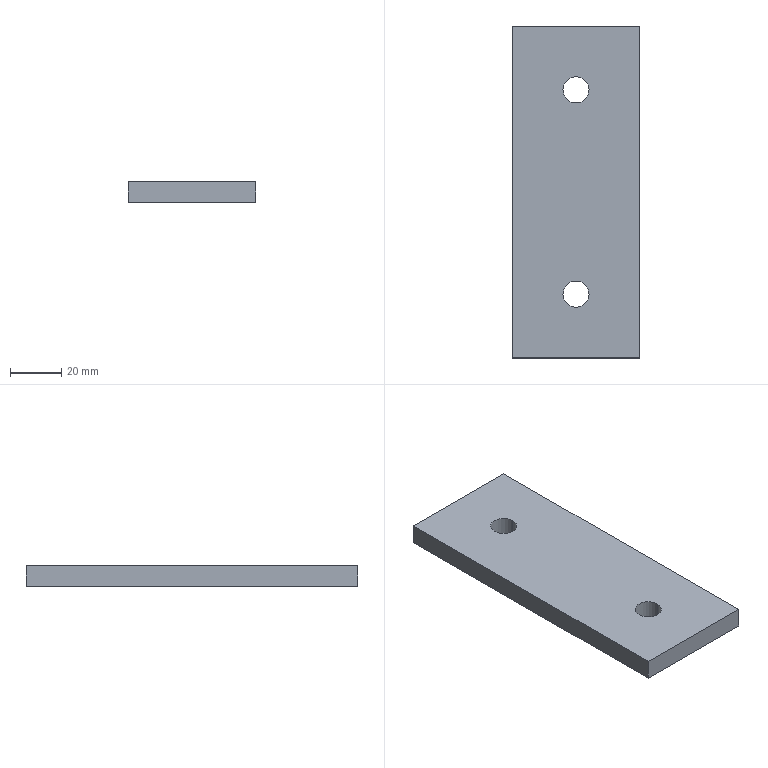Part | SolidWorks | features Extrusion 1, HoleWzd 1 | 1 solid | 10 faces | box 50 x 130 x 8 mm | volume 50693 mm3 | plane 6 | cylinder 4 | commonest cylinder face diameters 10.2 x4
STEP:
#1=CARTESIAN_POINT('',(-5.1,40.,0.));
#2=VERTEX_POINT('',#1);
#3=CARTESIAN_POINT('',(5.1,40.,0.));
#4=VERTEX_POINT('',#3);
#5=CARTESIAN_POINT('',(0.,40.,0.));
#6=DIRECTION('',(0.,0.,1.));
#7=DIRECTION('',(1.,0.,0.));
#8=AXIS2_PLACEMENT_3D('',#5,#6,#7);
#9=CIRCLE('',#8,5.1);
#10=EDGE_CURVE('',#2,#4,#9,.T.);
#11=ORIENTED_EDGE('',*,*,#10,.F.);
#12=CARTESIAN_POINT('',(-5.1,40.,8.));
#13=VERTEX_POINT('',#12);
#14=CARTESIAN_POINT('',(-5.1,40.,8.));
#15=DIRECTION('',(0.,0.,1.));
#16=VECTOR('',#15,1000.);
#17=LINE('',#14,#16);
#18=EDGE_CURVE('',#2,#13,#17,.T.);
#19=ORIENTED_EDGE('',*,*,#18,.T.);
#20=CARTESIAN_POINT('',(5.1,40.,8.));
#21=VERTEX_POINT('',#20);
#22=CARTESIAN_POINT('',(0.,40.,8.));
#23=DIRECTION('',(0.,0.,1.));
#24=DIRECTION('',(1.,0.,0.));
#25=AXIS2_PLACEMENT_3D('',#22,#23,#24);
#26=CIRCLE('',#25,5.1);
#27=EDGE_CURVE('',#13,#21,#26,.T.);
#28=ORIENTED_EDGE('',*,*,#27,.T.);
#29=CARTESIAN_POINT('',(5.1,40.,8.));
#30=DIRECTION('',(0.,0.,1.));
#31=VECTOR('',#30,1000.);
#32=LINE('',#29,#31);
#33=EDGE_CURVE('',#4,#21,#32,.T.);
#34=ORIENTED_EDGE('',*,*,#33,.F.);
#35=EDGE_LOOP('',(#11,#19,#28,#34));
#36=FACE_OUTER_BOUND('',#35,.T.);
#37=CARTESIAN_POINT('',(0.,40.,8.));
#38=DIRECTION('',(0.,0.,1.));
#39=DIRECTION('',(1.,0.,0.));
#40=AXIS2_PLACEMENT_3D('',#37,#38,#39);
#41=CYLINDRICAL_SURFACE('',#40,5.1);
#42=ADVANCED_FACE('',(#36),#41,.F.);
#43=CARTESIAN_POINT('',(-5.1,-40.,0.));
#44=VERTEX_POINT('',#43);
#45=CARTESIAN_POINT('',(5.1,-40.,0.));
#46=VERTEX_POINT('',#45);
#47=CARTESIAN_POINT('',(0.,-40.,0.));
#48=DIRECTION('',(0.,0.,1.));
#49=DIRECTION('',(1.,0.,0.));
#50=AXIS2_PLACEMENT_3D('',#47,#48,#49);
#51=CIRCLE('',#50,5.1);
#52=EDGE_CURVE('',#44,#46,#51,.T.);
#53=ORIENTED_EDGE('',*,*,#52,.F.);
#54=CARTESIAN_POINT('',(-5.1,-40.,8.));
#55=VERTEX_POINT('',#54);
#56=CARTESIAN_POINT('',(-5.1,-40.,8.));
#57=DIRECTION('',(0.,0.,1.));
#58=VECTOR('',#57,1000.);
#59=LINE('',#56,#58);
#60=EDGE_CURVE('',#44,#55,#59,.T.);
#61=ORIENTED_EDGE('',*,*,#60,.T.);
#62=CARTESIAN_POINT('',(5.1,-40.,8.));
#63=VERTEX_POINT('',#62);
#64=CARTESIAN_POINT('',(0.,-40.,8.));
#65=DIRECTION('',(0.,0.,1.));
#66=DIRECTION('',(1.,0.,0.));
#67=AXIS2_PLACEMENT_3D('',#64,#65,#66);
#68=CIRCLE('',#67,5.1);
#69=EDGE_CURVE('',#55,#63,#68,.T.);
#70=ORIENTED_EDGE('',*,*,#69,.T.);
#71=CARTESIAN_POINT('',(5.1,-40.,8.));
#72=DIRECTION('',(0.,0.,1.));
#73=VECTOR('',#72,1000.);
#74=LINE('',#71,#73);
#75=EDGE_CURVE('',#46,#63,#74,.T.);
#76=ORIENTED_EDGE('',*,*,#75,.F.);
#77=EDGE_LOOP('',(#53,#61,#70,#76));
#78=FACE_OUTER_BOUND('',#77,.T.);
#79=CARTESIAN_POINT('',(0.,-40.,8.));
#80=DIRECTION('',(0.,0.,1.));
#81=DIRECTION('',(1.,0.,0.));
#82=AXIS2_PLACEMENT_3D('',#79,#80,#81);
#83=CYLINDRICAL_SURFACE('',#82,5.1);
#84=ADVANCED_FACE('',(#78),#83,.F.);
#85=CARTESIAN_POINT('',(25.,-65.,0.));
#86=VERTEX_POINT('',#85);
#87=CARTESIAN_POINT('',(25.,65.,0.));
#88=VERTEX_POINT('',#87);
#89=CARTESIAN_POINT('',(25.,65.,0.));
#90=DIRECTION('',(0.,1.,0.));
#91=VECTOR('',#90,1000.);
#92=LINE('',#89,#91);
#93=EDGE_CURVE('',#86,#88,#92,.T.);
#94=ORIENTED_EDGE('',*,*,#93,.T.);
#95=CARTESIAN_POINT('',(25.,65.,8.));
#96=VERTEX_POINT('',#95);
#97=CARTESIAN_POINT('',(25.,65.,8.));
#98=DIRECTION('',(0.,0.,-1.));
#99=VECTOR('',#98,1000.);
#100=LINE('',#97,#99);
#101=EDGE_CURVE('',#96,#88,#100,.T.);
#102=ORIENTED_EDGE('',*,*,#101,.F.);
#103=CARTESIAN_POINT('',(25.,-65.,8.));
#104=VERTEX_POINT('',#103);
#105=CARTESIAN_POINT('',(25.,65.,8.));
#106=DIRECTION('',(0.,1.,0.));
#107=VECTOR('',#106,1000.);
#108=LINE('',#105,#107);
#109=EDGE_CURVE('',#104,#96,#108,.T.);
#110=ORIENTED_EDGE('',*,*,#109,.F.);
#111=CARTESIAN_POINT('',(25.,-65.,8.));
#112=DIRECTION('',(0.,0.,-1.));
#113=VECTOR('',#112,1000.);
#114=LINE('',#111,#113);
#115=EDGE_CURVE('',#104,#86,#114,.T.);
#116=ORIENTED_EDGE('',*,*,#115,.T.);
#117=EDGE_LOOP('',(#94,#102,#110,#116));
#118=FACE_OUTER_BOUND('',#117,.T.);
#119=CARTESIAN_POINT('',(25.,65.,8.));
#120=DIRECTION('',(-1.,0.,0.));
#121=DIRECTION('',(0.,-1.,0.));
#122=AXIS2_PLACEMENT_3D('',#119,#120,#121);
#123=PLANE('',#122);
#124=ADVANCED_FACE('',(#118),#123,.F.);
#125=CARTESIAN_POINT('',(-25.,65.,0.));
#126=VERTEX_POINT('',#125);
#127=CARTESIAN_POINT('',(-25.,65.,0.));
#128=DIRECTION('',(-1.,0.,0.));
#129=VECTOR('',#128,1000.);
#130=LINE('',#127,#129);
#131=EDGE_CURVE('',#88,#126,#130,.T.);
#132=ORIENTED_EDGE('',*,*,#131,.T.);
#133=CARTESIAN_POINT('',(-25.,65.,8.));
#134=VERTEX_POINT('',#133);
#135=CARTESIAN_POINT('',(-25.,65.,8.));
#136=DIRECTION('',(0.,0.,-1.));
#137=VECTOR('',#136,1000.);
#138=LINE('',#135,#137);
#139=EDGE_CURVE('',#134,#126,#138,.T.);
#140=ORIENTED_EDGE('',*,*,#139,.F.);
#141=CARTESIAN_POINT('',(-25.,65.,8.));
#142=DIRECTION('',(-1.,0.,0.));
#143=VECTOR('',#142,1000.);
#144=LINE('',#141,#143);
#145=EDGE_CURVE('',#96,#134,#144,.T.);
#146=ORIENTED_EDGE('',*,*,#145,.F.);
#147=ORIENTED_EDGE('',*,*,#101,.T.);
#148=EDGE_LOOP('',(#132,#140,#146,#147));
#149=FACE_OUTER_BOUND('',#148,.T.);
#150=CARTESIAN_POINT('',(-25.,65.,8.));
#151=DIRECTION('',(0.,-1.,0.));
#152=DIRECTION('',(0.,0.,-1.));
#153=AXIS2_PLACEMENT_3D('',#150,#151,#152);
#154=PLANE('',#153);
#155=ADVANCED_FACE('',(#149),#154,.F.);
#156=CARTESIAN_POINT('',(-25.,-65.,0.));
#157=VERTEX_POINT('',#156);
#158=CARTESIAN_POINT('',(-25.,65.,0.));
#159=DIRECTION('',(0.,-1.,0.));
#160=VECTOR('',#159,1000.);
#161=LINE('',#158,#160);
#162=EDGE_CURVE('',#126,#157,#161,.T.);
#163=ORIENTED_EDGE('',*,*,#162,.T.);
#164=CARTESIAN_POINT('',(-25.,-65.,8.));
#165=VERTEX_POINT('',#164);
#166=CARTESIAN_POINT('',(-25.,-65.,8.));
#167=DIRECTION('',(0.,0.,-1.));
#168=VECTOR('',#167,1000.);
#169=LINE('',#166,#168);
#170=EDGE_CURVE('',#165,#157,#169,.T.);
#171=ORIENTED_EDGE('',*,*,#170,.F.);
#172=CARTESIAN_POINT('',(-25.,65.,8.));
#173=DIRECTION('',(0.,-1.,0.));
#174=VECTOR('',#173,1000.);
#175=LINE('',#172,#174);
#176=EDGE_CURVE('',#134,#165,#175,.T.);
#177=ORIENTED_EDGE('',*,*,#176,.F.);
#178=ORIENTED_EDGE('',*,*,#139,.T.);
#179=EDGE_LOOP('',(#163,#171,#177,#178));
#180=FACE_OUTER_BOUND('',#179,.T.);
#181=CARTESIAN_POINT('',(-25.,65.,8.));
#182=DIRECTION('',(1.,0.,0.));
#183=DIRECTION('',(0.,1.,0.));
#184=AXIS2_PLACEMENT_3D('',#181,#182,#183);
#185=PLANE('',#184);
#186=ADVANCED_FACE('',(#180),#185,.F.);
#187=CARTESIAN_POINT('',(-25.,-65.,0.));
#188=DIRECTION('',(1.,0.,0.));
#189=VECTOR('',#188,1000.);
#190=LINE('',#187,#189);
#191=EDGE_CURVE('',#157,#86,#190,.T.);
#192=ORIENTED_EDGE('',*,*,#191,.T.);
#193=ORIENTED_EDGE('',*,*,#115,.F.);
#194=CARTESIAN_POINT('',(-25.,-65.,8.));
#195=DIRECTION('',(1.,0.,0.));
#196=VECTOR('',#195,1000.);
#197=LINE('',#194,#196);
#198=EDGE_CURVE('',#165,#104,#197,.T.);
#199=ORIENTED_EDGE('',*,*,#198,.F.);
#200=ORIENTED_EDGE('',*,*,#170,.T.);
#201=EDGE_LOOP('',(#192,#193,#199,#200));
#202=FACE_OUTER_BOUND('',#201,.T.);
#203=CARTESIAN_POINT('',(-25.,-65.,8.));
#204=DIRECTION('',(0.,1.,0.));
#205=DIRECTION('',(0.,0.,1.));
#206=AXIS2_PLACEMENT_3D('',#203,#204,#205);
#207=PLANE('',#206);
#208=ADVANCED_FACE('',(#202),#207,.F.);
#209=CARTESIAN_POINT('',(0.,40.,8.));
#210=DIRECTION('',(0.,0.,1.));
#211=DIRECTION('',(1.,0.,0.));
#212=AXIS2_PLACEMENT_3D('',#209,#210,#211);
#213=CIRCLE('',#212,5.1);
#214=EDGE_CURVE('',#21,#13,#213,.T.);
#215=ORIENTED_EDGE('',*,*,#214,.F.);
#216=ORIENTED_EDGE('',*,*,#27,.F.);
#217=EDGE_LOOP('',(#215,#216));
#218=FACE_BOUND('',#217,.T.);
#219=CARTESIAN_POINT('',(0.,-40.,8.));
#220=DIRECTION('',(0.,0.,1.));
#221=DIRECTION('',(1.,0.,0.));
#222=AXIS2_PLACEMENT_3D('',#219,#220,#221);
#223=CIRCLE('',#222,5.1);
#224=EDGE_CURVE('',#63,#55,#223,.T.);
#225=ORIENTED_EDGE('',*,*,#224,.F.);
#226=ORIENTED_EDGE('',*,*,#69,.F.);
#227=EDGE_LOOP('',(#225,#226));
#228=FACE_BOUND('',#227,.T.);
#229=ORIENTED_EDGE('',*,*,#109,.T.);
#230=ORIENTED_EDGE('',*,*,#145,.T.);
#231=ORIENTED_EDGE('',*,*,#176,.T.);
#232=ORIENTED_EDGE('',*,*,#198,.T.);
#233=EDGE_LOOP('',(#229,#230,#231,#232));
#234=FACE_OUTER_BOUND('',#233,.T.);
#235=CARTESIAN_POINT('',(0.,0.,8.));
#236=DIRECTION('',(0.,0.,1.));
#237=DIRECTION('',(1.,0.,0.));
#238=AXIS2_PLACEMENT_3D('',#235,#236,#237);
#239=PLANE('',#238);
#240=ADVANCED_FACE('',(#218,#228,#234),#239,.T.);
#241=CARTESIAN_POINT('',(0.,40.,0.));
#242=DIRECTION('',(0.,0.,1.));
#243=DIRECTION('',(1.,0.,0.));
#244=AXIS2_PLACEMENT_3D('',#241,#242,#243);
#245=CIRCLE('',#244,5.1);
#246=EDGE_CURVE('',#4,#2,#245,.T.);
#247=ORIENTED_EDGE('',*,*,#246,.T.);
#248=ORIENTED_EDGE('',*,*,#10,.T.);
#249=EDGE_LOOP('',(#247,#248));
#250=FACE_BOUND('',#249,.T.);
#251=CARTESIAN_POINT('',(0.,-40.,0.));
#252=DIRECTION('',(0.,0.,1.));
#253=DIRECTION('',(1.,0.,0.));
#254=AXIS2_PLACEMENT_3D('',#251,#252,#253);
#255=CIRCLE('',#254,5.1);
#256=EDGE_CURVE('',#46,#44,#255,.T.);
#257=ORIENTED_EDGE('',*,*,#256,.T.);
#258=ORIENTED_EDGE('',*,*,#52,.T.);
#259=EDGE_LOOP('',(#257,#258));
#260=FACE_BOUND('',#259,.T.);
#261=ORIENTED_EDGE('',*,*,#93,.F.);
#262=ORIENTED_EDGE('',*,*,#191,.F.);
#263=ORIENTED_EDGE('',*,*,#162,.F.);
#264=ORIENTED_EDGE('',*,*,#131,.F.);
#265=EDGE_LOOP('',(#261,#262,#263,#264));
#266=FACE_OUTER_BOUND('',#265,.T.);
#267=CARTESIAN_POINT('',(0.,0.,0.));
#268=DIRECTION('',(0.,0.,1.));
#269=DIRECTION('',(1.,0.,0.));
#270=AXIS2_PLACEMENT_3D('',#267,#268,#269);
#271=PLANE('',#270);
#272=ADVANCED_FACE('',(#250,#260,#266),#271,.F.);
#273=ORIENTED_EDGE('',*,*,#60,.F.);
#274=ORIENTED_EDGE('',*,*,#256,.F.);
#275=ORIENTED_EDGE('',*,*,#75,.T.);
#276=ORIENTED_EDGE('',*,*,#224,.T.);
#277=EDGE_LOOP('',(#273,#274,#275,#276));
#278=FACE_OUTER_BOUND('',#277,.T.);
#279=CARTESIAN_POINT('',(0.,-40.,8.));
#280=DIRECTION('',(0.,0.,1.));
#281=DIRECTION('',(1.,0.,0.));
#282=AXIS2_PLACEMENT_3D('',#279,#280,#281);
#283=CYLINDRICAL_SURFACE('',#282,5.1);
#284=ADVANCED_FACE('',(#278),#283,.F.);
#285=ORIENTED_EDGE('',*,*,#18,.F.);
#286=ORIENTED_EDGE('',*,*,#246,.F.);
#287=ORIENTED_EDGE('',*,*,#33,.T.);
#288=ORIENTED_EDGE('',*,*,#214,.T.);
#289=EDGE_LOOP('',(#285,#286,#287,#288));
#290=FACE_OUTER_BOUND('',#289,.T.);
#291=CARTESIAN_POINT('',(0.,40.,8.));
#292=DIRECTION('',(0.,0.,1.));
#293=DIRECTION('',(1.,0.,0.));
#294=AXIS2_PLACEMENT_3D('',#291,#292,#293);
#295=CYLINDRICAL_SURFACE('',#294,5.1);
#296=ADVANCED_FACE('',(#290),#295,.F.);
#297=CLOSED_SHELL('',(#42,#84,#124,#155,#186,#208,#240,#272,#284,#296));
#298=MANIFOLD_SOLID_BREP('',#297);
#299=CARTESIAN_POINT('',(0.,0.,0.));
#300=DIRECTION('',(0.,0.,1.));
#301=DIRECTION('',(1.,0.,0.));
#302=AXIS2_PLACEMENT_3D('',#299,#300,#301);
#303=(LENGTH_UNIT()NAMED_UNIT(*)SI_UNIT(.MILLI.,.METRE.));
#304=UNCERTAINTY_MEASURE_WITH_UNIT(LENGTH_MEASURE(0.00001),#303,'','');
#305=(NAMED_UNIT(*)PLANE_ANGLE_UNIT()SI_UNIT($,.RADIAN.));
#306=(NAMED_UNIT(*)SI_UNIT($,.STERADIAN.)SOLID_ANGLE_UNIT());
#307=(GEOMETRIC_REPRESENTATION_CONTEXT(3)GLOBAL_UNCERTAINTY_ASSIGNED_CONTEXT((#304))GLOBAL_UNIT_ASSIGNED_CONTEXT((#303,#305,#306))REPRESENTATION_CONTEXT('',''));
#308=ADVANCED_BREP_SHAPE_REPRESENTATION('',(#298,#302),#307);